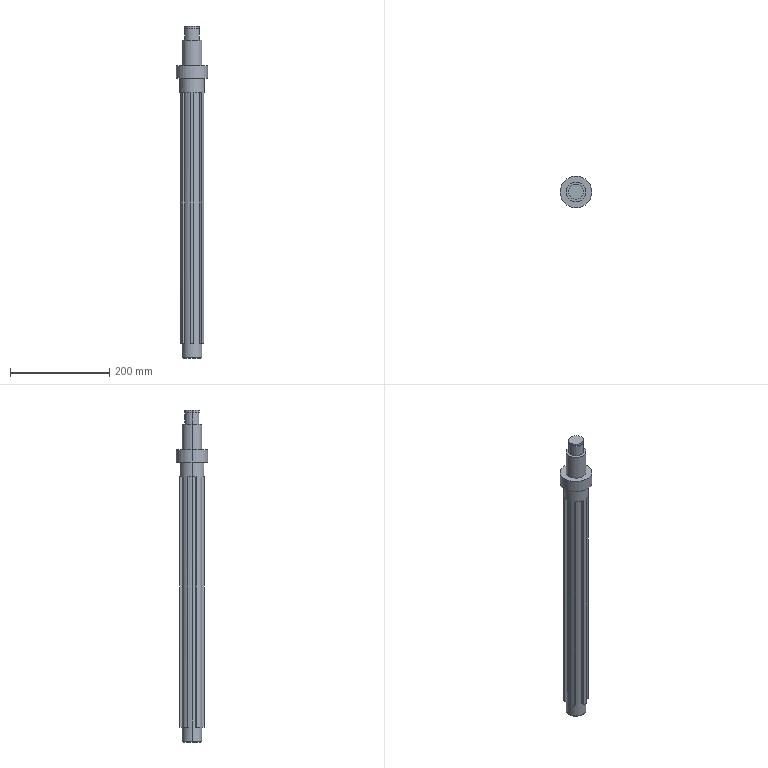Part | SolidWorks | features BaseBody 1 | 1 solid | 52 faces | box 64 x 64 x 670 mm | volume 1017560 mm3 | plane 34 | cylinder 16 | cone 2 | commonest cylinder face diameters 30 x4 40 x4 8 x2 27.9 x2 50 x2 64 x2